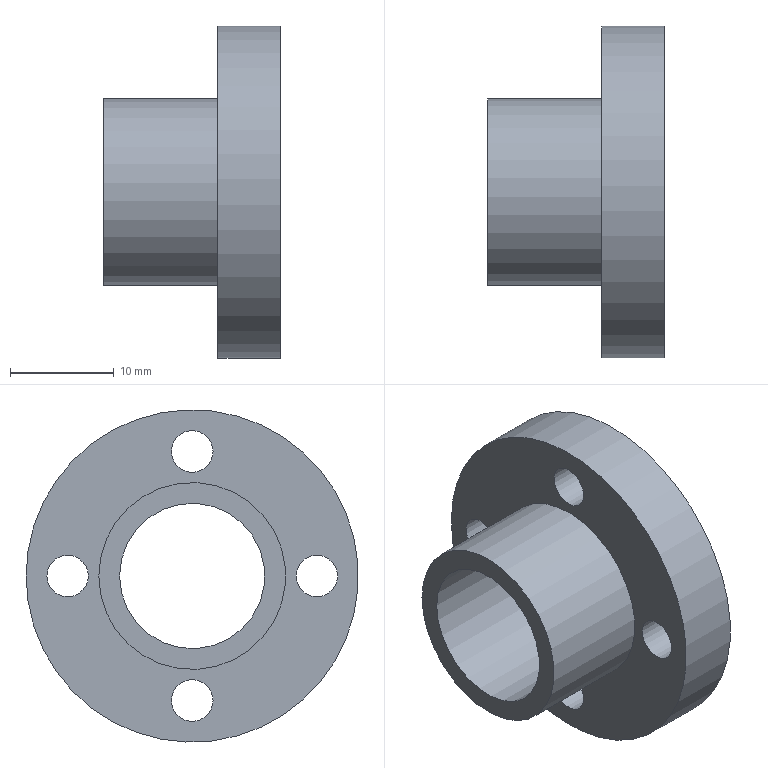Part | STEP file | 1-56.13 | 1 solid | 10 faces | box 17 x 32 x 32 mm | volume 4706 mm3 | cylinder 7 | plane 3 | commonest cylinder face diameters 4 x4 14 x1 18 x1 32 x1
STEP:
#1=CARTESIAN_POINT('',(0.,0.,0.));
#2=DIRECTION('',(0.,0.,1.));
#3=DIRECTION('',(1.,0.,0.));
#4=AXIS2_PLACEMENT_3D('',#1,#2,#3);
#5=CARTESIAN_POINT('',(-11.,9.,0.));
#6=VERTEX_POINT('',#5);
#7=CARTESIAN_POINT('',(-11.,0.,0.));
#8=DIRECTION('',(1.,0.,0.));
#9=DIRECTION('',(0.,1.,0.));
#10=AXIS2_PLACEMENT_3D('',#7,#8,#9);
#11=CIRCLE('',#10,9.);
#12=CARTESIAN_POINT('',(-11.,-2.412,0.));
#13=DIRECTION('',(1.,0.,0.));
#14=DIRECTION('',(0.,0.,-1.));
#15=AXIS2_PLACEMENT_3D('',#12,#13,#14);
#16=PLANE('',#15);
#17=CARTESIAN_POINT('',(0.,2.412));
#18=DIRECTION('',(0.,1.));
#19=AXIS2_PLACEMENT_2D('',#17,#18);
#20=CIRCLE('',#19,9.);
#21=(GEOMETRIC_REPRESENTATION_CONTEXT(2)PARAMETRIC_REPRESENTATION_CONTEXT()REPRESENTATION_CONTEXT('',''));
#22=DEFINITIONAL_REPRESENTATION('',(#20),#21);
#23=PCURVE('',#16,#22);
#24=CARTESIAN_POINT('',(0.,0.,0.));
#25=DIRECTION('',(-1.,0.,0.));
#26=DIRECTION('',(0.,1.,0.));
#27=AXIS2_PLACEMENT_3D('',#24,#25,#26);
#28=CYLINDRICAL_SURFACE('',#27,9.);
#29=CARTESIAN_POINT('',(6.283,11.));
#30=DIRECTION('',(-1.,0.));
#31=VECTOR('',#30,1.);
#32=LINE('',#29,#31);
#33=(GEOMETRIC_REPRESENTATION_CONTEXT(2)PARAMETRIC_REPRESENTATION_CONTEXT()REPRESENTATION_CONTEXT('',''));
#34=DEFINITIONAL_REPRESENTATION('',(#32),#33);
#35=PCURVE('',#28,#34);
#36=SURFACE_CURVE('',#11,(#23,#35),.PCURVE_S1.);
#37=EDGE_CURVE('',#6,#6,#36,.T.);
#38=ORIENTED_EDGE('',*,*,#37,.T.);
#39=EDGE_LOOP('',(#38));
#40=FACE_BOUND('',#39,.F.);
#41=CARTESIAN_POINT('',(-11.,7.,0.));
#42=VERTEX_POINT('',#41);
#43=CARTESIAN_POINT('',(-11.,0.,0.));
#44=DIRECTION('',(-1.,0.,0.));
#45=DIRECTION('',(0.,1.,0.));
#46=AXIS2_PLACEMENT_3D('',#43,#44,#45);
#47=CIRCLE('',#46,7.);
#48=CARTESIAN_POINT('',(0.,9.412));
#49=CARTESIAN_POINT('',(12.124,9.412));
#50=CARTESIAN_POINT('',(6.062,-1.088));
#51=CARTESIAN_POINT('',(0.,-11.588));
#52=CARTESIAN_POINT('',(-6.062,-1.088));
#53=CARTESIAN_POINT('',(-12.124,9.412));
#54=CARTESIAN_POINT('',(0.,9.412));
#55=(BOUNDED_CURVE()B_SPLINE_CURVE(2,(#48,#49,#50,#51,#52,#53,#54),.UNSPECIFIED.,.T.,.F.)B_SPLINE_CURVE_WITH_KNOTS((1,2,2,2,2,1),(-2.094,0.,2.094,4.189,6.283,8.378),.UNSPECIFIED.)CURVE()GEOMETRIC_REPRESENTATION_ITEM()RATIONAL_B_SPLINE_CURVE((1.,0.5,1.,0.5,1.,0.5,1.))REPRESENTATION_ITEM(''));
#56=(GEOMETRIC_REPRESENTATION_CONTEXT(2)PARAMETRIC_REPRESENTATION_CONTEXT()REPRESENTATION_CONTEXT('',''));
#57=DEFINITIONAL_REPRESENTATION('',(#55),#56);
#58=PCURVE('',#16,#57);
#59=CARTESIAN_POINT('',(6.,0.,0.));
#60=DIRECTION('',(-1.,0.,0.));
#61=DIRECTION('',(0.,1.,0.));
#62=AXIS2_PLACEMENT_3D('',#59,#60,#61);
#63=CYLINDRICAL_SURFACE('',#62,7.);
#64=CARTESIAN_POINT('',(0.,17.));
#65=DIRECTION('',(1.,0.));
#66=VECTOR('',#65,1.);
#67=LINE('',#64,#66);
#68=(GEOMETRIC_REPRESENTATION_CONTEXT(2)PARAMETRIC_REPRESENTATION_CONTEXT()REPRESENTATION_CONTEXT('',''));
#69=DEFINITIONAL_REPRESENTATION('',(#67),#68);
#70=PCURVE('',#63,#69);
#71=SURFACE_CURVE('',#47,(#58,#70),.PCURVE_S1.);
#72=EDGE_CURVE('',#42,#42,#71,.T.);
#73=ORIENTED_EDGE('',*,*,#72,.T.);
#74=EDGE_LOOP('',(#73));
#75=FACE_BOUND('',#74,.F.);
#76=ADVANCED_FACE('',(#40,#75),#16,.F.);
#77=CARTESIAN_POINT('',(0.,9.,0.));
#78=VERTEX_POINT('',#77);
#79=CARTESIAN_POINT('',(0.,9.,0.));
#80=DIRECTION('',(-1.,0.,0.));
#81=VECTOR('',#80,1.);
#82=LINE('',#79,#81);
#83=CARTESIAN_POINT('',(6.283,0.));
#84=DIRECTION('',(0.,1.));
#85=VECTOR('',#84,1.);
#86=LINE('',#83,#85);
#87=(GEOMETRIC_REPRESENTATION_CONTEXT(2)PARAMETRIC_REPRESENTATION_CONTEXT()REPRESENTATION_CONTEXT('',''));
#88=DEFINITIONAL_REPRESENTATION('',(#86),#87);
#89=PCURVE('',#28,#88);
#90=CARTESIAN_POINT('',(0.,0.));
#91=DIRECTION('',(0.,1.));
#92=VECTOR('',#91,1.);
#93=LINE('',#90,#92);
#94=(GEOMETRIC_REPRESENTATION_CONTEXT(2)PARAMETRIC_REPRESENTATION_CONTEXT()REPRESENTATION_CONTEXT('',''));
#95=DEFINITIONAL_REPRESENTATION('',(#93),#94);
#96=PCURVE('',#28,#95);
#97=SEAM_CURVE('',#82,(#89,#96),.PCURVE_S1.);
#98=EDGE_CURVE('',#78,#6,#97,.T.);
#99=ORIENTED_EDGE('',*,*,#98,.T.);
#100=ORIENTED_EDGE('',*,*,#37,.T.);
#101=ORIENTED_EDGE('',*,*,#98,.F.);
#102=CARTESIAN_POINT('',(0.,0.,0.));
#103=DIRECTION('',(1.,0.,0.));
#104=DIRECTION('',(0.,1.,0.));
#105=AXIS2_PLACEMENT_3D('',#102,#103,#104);
#106=CIRCLE('',#105,9.);
#107=CARTESIAN_POINT('',(6.283,0.));
#108=DIRECTION('',(-1.,0.));
#109=VECTOR('',#108,1.);
#110=LINE('',#107,#109);
#111=(GEOMETRIC_REPRESENTATION_CONTEXT(2)PARAMETRIC_REPRESENTATION_CONTEXT()REPRESENTATION_CONTEXT('',''));
#112=DEFINITIONAL_REPRESENTATION('',(#110),#111);
#113=PCURVE('',#28,#112);
#114=CARTESIAN_POINT('',(0.,-4.287,0.));
#115=DIRECTION('',(1.,0.,0.));
#116=DIRECTION('',(0.,0.,-1.));
#117=AXIS2_PLACEMENT_3D('',#114,#115,#116);
#118=PLANE('',#117);
#119=CARTESIAN_POINT('',(0.,4.287));
#120=DIRECTION('',(0.,1.));
#121=AXIS2_PLACEMENT_2D('',#119,#120);
#122=CIRCLE('',#121,9.);
#123=(GEOMETRIC_REPRESENTATION_CONTEXT(2)PARAMETRIC_REPRESENTATION_CONTEXT()REPRESENTATION_CONTEXT('',''));
#124=DEFINITIONAL_REPRESENTATION('',(#122),#123);
#125=PCURVE('',#118,#124);
#126=SURFACE_CURVE('',#106,(#113,#125),.PCURVE_S1.);
#127=EDGE_CURVE('',#78,#78,#126,.T.);
#128=ORIENTED_EDGE('',*,*,#127,.F.);
#129=EDGE_LOOP('',(#99,#100,#101,#128));
#130=FACE_BOUND('',#129,.T.);
#131=ADVANCED_FACE('',(#130),#28,.T.);
#132=ORIENTED_EDGE('',*,*,#72,.F.);
#133=CARTESIAN_POINT('',(6.,7.,0.));
#134=VERTEX_POINT('',#133);
#135=CARTESIAN_POINT('',(-11.,7.,0.));
#136=DIRECTION('',(1.,0.,0.));
#137=VECTOR('',#136,1.);
#138=LINE('',#135,#137);
#139=CARTESIAN_POINT('',(0.,17.));
#140=DIRECTION('',(0.,-1.));
#141=VECTOR('',#140,1.);
#142=LINE('',#139,#141);
#143=(GEOMETRIC_REPRESENTATION_CONTEXT(2)PARAMETRIC_REPRESENTATION_CONTEXT()REPRESENTATION_CONTEXT('',''));
#144=DEFINITIONAL_REPRESENTATION('',(#142),#143);
#145=PCURVE('',#63,#144);
#146=CARTESIAN_POINT('',(6.283,17.));
#147=DIRECTION('',(0.,-1.));
#148=VECTOR('',#147,1.);
#149=LINE('',#146,#148);
#150=(GEOMETRIC_REPRESENTATION_CONTEXT(2)PARAMETRIC_REPRESENTATION_CONTEXT()REPRESENTATION_CONTEXT('',''));
#151=DEFINITIONAL_REPRESENTATION('',(#149),#150);
#152=PCURVE('',#63,#151);
#153=SEAM_CURVE('',#138,(#145,#152),.PCURVE_S1.);
#154=EDGE_CURVE('',#42,#134,#153,.T.);
#155=ORIENTED_EDGE('',*,*,#154,.T.);
#156=CARTESIAN_POINT('',(6.,0.,0.));
#157=DIRECTION('',(-1.,0.,0.));
#158=DIRECTION('',(0.,1.,0.));
#159=AXIS2_PLACEMENT_3D('',#156,#157,#158);
#160=CIRCLE('',#159,7.);
#161=CARTESIAN_POINT('',(0.,0.));
#162=DIRECTION('',(1.,0.));
#163=VECTOR('',#162,1.);
#164=LINE('',#161,#163);
#165=(GEOMETRIC_REPRESENTATION_CONTEXT(2)PARAMETRIC_REPRESENTATION_CONTEXT()REPRESENTATION_CONTEXT('',''));
#166=DEFINITIONAL_REPRESENTATION('',(#164),#165);
#167=PCURVE('',#63,#166);
#168=CARTESIAN_POINT('',(6.,-4.287,0.));
#169=DIRECTION('',(1.,0.,0.));
#170=DIRECTION('',(0.,0.,-1.));
#171=AXIS2_PLACEMENT_3D('',#168,#169,#170);
#172=PLANE('',#171);
#173=CARTESIAN_POINT('',(0.,11.287));
#174=CARTESIAN_POINT('',(12.124,11.287));
#175=CARTESIAN_POINT('',(6.062,0.7872));
#176=CARTESIAN_POINT('',(0.,-9.713));
#177=CARTESIAN_POINT('',(-6.062,0.7872));
#178=CARTESIAN_POINT('',(-12.124,11.287));
#179=CARTESIAN_POINT('',(0.,11.287));
#180=(BOUNDED_CURVE()B_SPLINE_CURVE(2,(#173,#174,#175,#176,#177,#178,#179),.UNSPECIFIED.,.T.,.F.)B_SPLINE_CURVE_WITH_KNOTS((1,2,2,2,2,1),(-2.094,0.,2.094,4.189,6.283,8.378),.UNSPECIFIED.)CURVE()GEOMETRIC_REPRESENTATION_ITEM()RATIONAL_B_SPLINE_CURVE((1.,0.5,1.,0.5,1.,0.5,1.))REPRESENTATION_ITEM(''));
#181=(GEOMETRIC_REPRESENTATION_CONTEXT(2)PARAMETRIC_REPRESENTATION_CONTEXT()REPRESENTATION_CONTEXT('',''));
#182=DEFINITIONAL_REPRESENTATION('',(#180),#181);
#183=PCURVE('',#172,#182);
#184=SURFACE_CURVE('',#160,(#167,#183),.PCURVE_S1.);
#185=EDGE_CURVE('',#134,#134,#184,.T.);
#186=ORIENTED_EDGE('',*,*,#185,.T.);
#187=ORIENTED_EDGE('',*,*,#154,.F.);
#188=EDGE_LOOP('',(#132,#155,#186,#187));
#189=FACE_BOUND('',#188,.F.);
#190=ADVANCED_FACE('',(#189),#63,.F.);
#191=CARTESIAN_POINT('',(0.,16.,0.));
#192=VERTEX_POINT('',#191);
#193=CARTESIAN_POINT('',(0.,0.,0.));
#194=DIRECTION('',(1.,0.,0.));
#195=DIRECTION('',(0.,1.,0.));
#196=AXIS2_PLACEMENT_3D('',#193,#194,#195);
#197=CIRCLE('',#196,16.);
#198=CARTESIAN_POINT('',(0.,4.287));
#199=DIRECTION('',(0.,1.));
#200=AXIS2_PLACEMENT_2D('',#198,#199);
#201=CIRCLE('',#200,16.);
#202=(GEOMETRIC_REPRESENTATION_CONTEXT(2)PARAMETRIC_REPRESENTATION_CONTEXT()REPRESENTATION_CONTEXT('',''));
#203=DEFINITIONAL_REPRESENTATION('',(#201),#202);
#204=PCURVE('',#118,#203);
#205=CARTESIAN_POINT('',(0.,0.,0.));
#206=DIRECTION('',(1.,0.,0.));
#207=DIRECTION('',(0.,1.,0.));
#208=AXIS2_PLACEMENT_3D('',#205,#206,#207);
#209=CYLINDRICAL_SURFACE('',#208,16.);
#210=CARTESIAN_POINT('',(0.,0.));
#211=DIRECTION('',(1.,0.));
#212=VECTOR('',#211,1.);
#213=LINE('',#210,#212);
#214=(GEOMETRIC_REPRESENTATION_CONTEXT(2)PARAMETRIC_REPRESENTATION_CONTEXT()REPRESENTATION_CONTEXT('',''));
#215=DEFINITIONAL_REPRESENTATION('',(#213),#214);
#216=PCURVE('',#209,#215);
#217=SURFACE_CURVE('',#197,(#204,#216),.PCURVE_S1.);
#218=EDGE_CURVE('',#192,#192,#217,.T.);
#219=ORIENTED_EDGE('',*,*,#218,.T.);
#220=EDGE_LOOP('',(#219));
#221=FACE_BOUND('',#220,.F.);
#222=ORIENTED_EDGE('',*,*,#127,.F.);
#223=EDGE_LOOP('',(#222));
#224=FACE_BOUND('',#223,.F.);
#225=CARTESIAN_POINT('',(0.,2.,-12.));
#226=VERTEX_POINT('',#225);
#227=CARTESIAN_POINT('',(0.,0.,-12.));
#228=DIRECTION('',(-1.,0.,0.));
#229=DIRECTION('',(0.,1.,0.));
#230=AXIS2_PLACEMENT_3D('',#227,#228,#229);
#231=CIRCLE('',#230,2.);
#232=CARTESIAN_POINT('',(12.,6.287));
#233=CARTESIAN_POINT('',(15.464,6.287));
#234=CARTESIAN_POINT('',(13.732,3.287));
#235=CARTESIAN_POINT('',(12.,0.2872));
#236=CARTESIAN_POINT('',(10.268,3.287));
#237=CARTESIAN_POINT('',(8.536,6.287));
#238=CARTESIAN_POINT('',(12.,6.287));
#239=(BOUNDED_CURVE()B_SPLINE_CURVE(2,(#232,#233,#234,#235,#236,#237,#238),.UNSPECIFIED.,.T.,.F.)B_SPLINE_CURVE_WITH_KNOTS((1,2,2,2,2,1),(-2.094,0.,2.094,4.189,6.283,8.378),.UNSPECIFIED.)CURVE()GEOMETRIC_REPRESENTATION_ITEM()RATIONAL_B_SPLINE_CURVE((1.,0.5,1.,0.5,1.,0.5,1.))REPRESENTATION_ITEM(''));
#240=(GEOMETRIC_REPRESENTATION_CONTEXT(2)PARAMETRIC_REPRESENTATION_CONTEXT()REPRESENTATION_CONTEXT('',''));
#241=DEFINITIONAL_REPRESENTATION('',(#239),#240);
#242=PCURVE('',#118,#241);
#243=CARTESIAN_POINT('',(0.,0.,-12.));
#244=DIRECTION('',(1.,0.,0.));
#245=DIRECTION('',(0.,1.,0.));
#246=AXIS2_PLACEMENT_3D('',#243,#244,#245);
#247=CYLINDRICAL_SURFACE('',#246,2.);
#248=CARTESIAN_POINT('',(6.283,0.));
#249=DIRECTION('',(-1.,0.));
#250=VECTOR('',#249,1.);
#251=LINE('',#248,#250);
#252=(GEOMETRIC_REPRESENTATION_CONTEXT(2)PARAMETRIC_REPRESENTATION_CONTEXT()REPRESENTATION_CONTEXT('',''));
#253=DEFINITIONAL_REPRESENTATION('',(#251),#252);
#254=PCURVE('',#247,#253);
#255=SURFACE_CURVE('',#231,(#242,#254),.PCURVE_S1.);
#256=EDGE_CURVE('',#226,#226,#255,.T.);
#257=ORIENTED_EDGE('',*,*,#256,.T.);
#258=EDGE_LOOP('',(#257));
#259=FACE_BOUND('',#258,.F.);
#260=CARTESIAN_POINT('',(0.,2.,12.));
#261=VERTEX_POINT('',#260);
#262=CARTESIAN_POINT('',(0.,0.,12.));
#263=DIRECTION('',(-1.,0.,0.));
#264=DIRECTION('',(0.,1.,0.));
#265=AXIS2_PLACEMENT_3D('',#262,#263,#264);
#266=CIRCLE('',#265,2.);
#267=CARTESIAN_POINT('',(-12.,6.287));
#268=CARTESIAN_POINT('',(-8.536,6.287));
#269=CARTESIAN_POINT('',(-10.268,3.287));
#270=CARTESIAN_POINT('',(-12.,0.2872));
#271=CARTESIAN_POINT('',(-13.732,3.287));
#272=CARTESIAN_POINT('',(-15.464,6.287));
#273=CARTESIAN_POINT('',(-12.,6.287));
#274=(BOUNDED_CURVE()B_SPLINE_CURVE(2,(#267,#268,#269,#270,#271,#272,#273),.UNSPECIFIED.,.T.,.F.)B_SPLINE_CURVE_WITH_KNOTS((1,2,2,2,2,1),(-2.094,0.,2.094,4.189,6.283,8.378),.UNSPECIFIED.)CURVE()GEOMETRIC_REPRESENTATION_ITEM()RATIONAL_B_SPLINE_CURVE((1.,0.5,1.,0.5,1.,0.5,1.))REPRESENTATION_ITEM(''));
#275=(GEOMETRIC_REPRESENTATION_CONTEXT(2)PARAMETRIC_REPRESENTATION_CONTEXT()REPRESENTATION_CONTEXT('',''));
#276=DEFINITIONAL_REPRESENTATION('',(#274),#275);
#277=PCURVE('',#118,#276);
#278=CARTESIAN_POINT('',(0.,0.,12.));
#279=DIRECTION('',(1.,0.,0.));
#280=DIRECTION('',(0.,1.,0.));
#281=AXIS2_PLACEMENT_3D('',#278,#279,#280);
#282=CYLINDRICAL_SURFACE('',#281,2.);
#283=CARTESIAN_POINT('',(6.283,0.));
#284=DIRECTION('',(-1.,0.));
#285=VECTOR('',#284,1.);
#286=LINE('',#283,#285);
#287=(GEOMETRIC_REPRESENTATION_CONTEXT(2)PARAMETRIC_REPRESENTATION_CONTEXT()REPRESENTATION_CONTEXT('',''));
#288=DEFINITIONAL_REPRESENTATION('',(#286),#287);
#289=PCURVE('',#282,#288);
#290=SURFACE_CURVE('',#266,(#277,#289),.PCURVE_S1.);
#291=EDGE_CURVE('',#261,#261,#290,.T.);
#292=ORIENTED_EDGE('',*,*,#291,.T.);
#293=EDGE_LOOP('',(#292));
#294=FACE_BOUND('',#293,.F.);
#295=CARTESIAN_POINT('',(0.,14.,0.));
#296=VERTEX_POINT('',#295);
#297=CARTESIAN_POINT('',(0.,12.,0.));
#298=DIRECTION('',(-1.,0.,0.));
#299=DIRECTION('',(0.,1.,0.));
#300=AXIS2_PLACEMENT_3D('',#297,#298,#299);
#301=CIRCLE('',#300,2.);
#302=CARTESIAN_POINT('',(0.,18.287));
#303=CARTESIAN_POINT('',(3.464,18.287));
#304=CARTESIAN_POINT('',(1.732,15.287));
#305=CARTESIAN_POINT('',(0.,12.287));
#306=CARTESIAN_POINT('',(-1.732,15.287));
#307=CARTESIAN_POINT('',(-3.464,18.287));
#308=CARTESIAN_POINT('',(0.,18.287));
#309=(BOUNDED_CURVE()B_SPLINE_CURVE(2,(#302,#303,#304,#305,#306,#307,#308),.UNSPECIFIED.,.T.,.F.)B_SPLINE_CURVE_WITH_KNOTS((1,2,2,2,2,1),(-2.094,0.,2.094,4.189,6.283,8.378),.UNSPECIFIED.)CURVE()GEOMETRIC_REPRESENTATION_ITEM()RATIONAL_B_SPLINE_CURVE((1.,0.5,1.,0.5,1.,0.5,1.))REPRESENTATION_ITEM(''));
#310=(GEOMETRIC_REPRESENTATION_CONTEXT(2)PARAMETRIC_REPRESENTATION_CONTEXT()REPRESENTATION_CONTEXT('',''));
#311=DEFINITIONAL_REPRESENTATION('',(#309),#310);
#312=PCURVE('',#118,#311);
#313=CARTESIAN_POINT('',(0.,12.,0.));
#314=DIRECTION('',(1.,0.,0.));
#315=DIRECTION('',(0.,1.,0.));
#316=AXIS2_PLACEMENT_3D('',#313,#314,#315);
#317=CYLINDRICAL_SURFACE('',#316,2.);
#318=CARTESIAN_POINT('',(6.283,0.));
#319=DIRECTION('',(-1.,0.));
#320=VECTOR('',#319,1.);
#321=LINE('',#318,#320);
#322=(GEOMETRIC_REPRESENTATION_CONTEXT(2)PARAMETRIC_REPRESENTATION_CONTEXT()REPRESENTATION_CONTEXT('',''));
#323=DEFINITIONAL_REPRESENTATION('',(#321),#322);
#324=PCURVE('',#317,#323);
#325=SURFACE_CURVE('',#301,(#312,#324),.PCURVE_S1.);
#326=EDGE_CURVE('',#296,#296,#325,.T.);
#327=ORIENTED_EDGE('',*,*,#326,.T.);
#328=EDGE_LOOP('',(#327));
#329=FACE_BOUND('',#328,.F.);
#330=CARTESIAN_POINT('',(0.,-10.,0.));
#331=VERTEX_POINT('',#330);
#332=CARTESIAN_POINT('',(0.,-12.,0.));
#333=DIRECTION('',(-1.,0.,0.));
#334=DIRECTION('',(0.,1.,0.));
#335=AXIS2_PLACEMENT_3D('',#332,#333,#334);
#336=CIRCLE('',#335,2.);
#337=CARTESIAN_POINT('',(0.,-5.713));
#338=CARTESIAN_POINT('',(3.464,-5.713));
#339=CARTESIAN_POINT('',(1.732,-8.713));
#340=CARTESIAN_POINT('',(0.,-11.713));
#341=CARTESIAN_POINT('',(-1.732,-8.713));
#342=CARTESIAN_POINT('',(-3.464,-5.713));
#343=CARTESIAN_POINT('',(0.,-5.713));
#344=(BOUNDED_CURVE()B_SPLINE_CURVE(2,(#337,#338,#339,#340,#341,#342,#343),.UNSPECIFIED.,.T.,.F.)B_SPLINE_CURVE_WITH_KNOTS((1,2,2,2,2,1),(-2.094,0.,2.094,4.189,6.283,8.378),.UNSPECIFIED.)CURVE()GEOMETRIC_REPRESENTATION_ITEM()RATIONAL_B_SPLINE_CURVE((1.,0.5,1.,0.5,1.,0.5,1.))REPRESENTATION_ITEM(''));
#345=(GEOMETRIC_REPRESENTATION_CONTEXT(2)PARAMETRIC_REPRESENTATION_CONTEXT()REPRESENTATION_CONTEXT('',''));
#346=DEFINITIONAL_REPRESENTATION('',(#344),#345);
#347=PCURVE('',#118,#346);
#348=CARTESIAN_POINT('',(0.,-12.,0.));
#349=DIRECTION('',(1.,0.,0.));
#350=DIRECTION('',(0.,1.,0.));
#351=AXIS2_PLACEMENT_3D('',#348,#349,#350);
#352=CYLINDRICAL_SURFACE('',#351,2.);
#353=CARTESIAN_POINT('',(6.283,0.));
#354=DIRECTION('',(-1.,0.));
#355=VECTOR('',#354,1.);
#356=LINE('',#353,#355);
#357=(GEOMETRIC_REPRESENTATION_CONTEXT(2)PARAMETRIC_REPRESENTATION_CONTEXT()REPRESENTATION_CONTEXT('',''));
#358=DEFINITIONAL_REPRESENTATION('',(#356),#357);
#359=PCURVE('',#352,#358);
#360=SURFACE_CURVE('',#336,(#347,#359),.PCURVE_S1.);
#361=EDGE_CURVE('',#331,#331,#360,.T.);
#362=ORIENTED_EDGE('',*,*,#361,.T.);
#363=EDGE_LOOP('',(#362));
#364=FACE_BOUND('',#363,.F.);
#365=ADVANCED_FACE('',(#221,#224,#259,#294,#329,#364),#118,.F.);
#366=ORIENTED_EDGE('',*,*,#218,.T.);
#367=CARTESIAN_POINT('',(6.,16.,0.));
#368=VERTEX_POINT('',#367);
#369=CARTESIAN_POINT('',(0.,16.,0.));
#370=DIRECTION('',(1.,0.,0.));
#371=VECTOR('',#370,1.);
#372=LINE('',#369,#371);
#373=CARTESIAN_POINT('',(6.283,0.));
#374=DIRECTION('',(0.,1.));
#375=VECTOR('',#374,1.);
#376=LINE('',#373,#375);
#377=(GEOMETRIC_REPRESENTATION_CONTEXT(2)PARAMETRIC_REPRESENTATION_CONTEXT()REPRESENTATION_CONTEXT('',''));
#378=DEFINITIONAL_REPRESENTATION('',(#376),#377);
#379=PCURVE('',#209,#378);
#380=CARTESIAN_POINT('',(0.,0.));
#381=DIRECTION('',(0.,1.));
#382=VECTOR('',#381,1.);
#383=LINE('',#380,#382);
#384=(GEOMETRIC_REPRESENTATION_CONTEXT(2)PARAMETRIC_REPRESENTATION_CONTEXT()REPRESENTATION_CONTEXT('',''));
#385=DEFINITIONAL_REPRESENTATION('',(#383),#384);
#386=PCURVE('',#209,#385);
#387=SEAM_CURVE('',#372,(#379,#386),.PCURVE_S1.);
#388=EDGE_CURVE('',#192,#368,#387,.T.);
#389=ORIENTED_EDGE('',*,*,#388,.T.);
#390=CARTESIAN_POINT('',(6.,0.,0.));
#391=DIRECTION('',(1.,0.,0.));
#392=DIRECTION('',(0.,1.,0.));
#393=AXIS2_PLACEMENT_3D('',#390,#391,#392);
#394=CIRCLE('',#393,16.);
#395=CARTESIAN_POINT('',(0.,6.));
#396=DIRECTION('',(1.,0.));
#397=VECTOR('',#396,1.);
#398=LINE('',#395,#397);
#399=(GEOMETRIC_REPRESENTATION_CONTEXT(2)PARAMETRIC_REPRESENTATION_CONTEXT()REPRESENTATION_CONTEXT('',''));
#400=DEFINITIONAL_REPRESENTATION('',(#398),#399);
#401=PCURVE('',#209,#400);
#402=CARTESIAN_POINT('',(0.,4.287));
#403=DIRECTION('',(0.,1.));
#404=AXIS2_PLACEMENT_2D('',#402,#403);
#405=CIRCLE('',#404,16.);
#406=(GEOMETRIC_REPRESENTATION_CONTEXT(2)PARAMETRIC_REPRESENTATION_CONTEXT()REPRESENTATION_CONTEXT('',''));
#407=DEFINITIONAL_REPRESENTATION('',(#405),#406);
#408=PCURVE('',#172,#407);
#409=SURFACE_CURVE('',#394,(#401,#408),.PCURVE_S1.);
#410=EDGE_CURVE('',#368,#368,#409,.T.);
#411=ORIENTED_EDGE('',*,*,#410,.F.);
#412=ORIENTED_EDGE('',*,*,#388,.F.);
#413=EDGE_LOOP('',(#366,#389,#411,#412));
#414=FACE_BOUND('',#413,.T.);
#415=ADVANCED_FACE('',(#414),#209,.T.);
#416=CARTESIAN_POINT('',(6.,2.,-12.));
#417=VERTEX_POINT('',#416);
#418=CARTESIAN_POINT('',(0.,2.,-12.));
#419=DIRECTION('',(1.,0.,0.));
#420=VECTOR('',#419,1.);
#421=LINE('',#418,#420);
#422=CARTESIAN_POINT('',(6.283,0.));
#423=DIRECTION('',(0.,1.));
#424=VECTOR('',#423,1.);
#425=LINE('',#422,#424);
#426=(GEOMETRIC_REPRESENTATION_CONTEXT(2)PARAMETRIC_REPRESENTATION_CONTEXT()REPRESENTATION_CONTEXT('',''));
#427=DEFINITIONAL_REPRESENTATION('',(#425),#426);
#428=PCURVE('',#247,#427);
#429=CARTESIAN_POINT('',(0.,0.));
#430=DIRECTION('',(0.,1.));
#431=VECTOR('',#430,1.);
#432=LINE('',#429,#431);
#433=(GEOMETRIC_REPRESENTATION_CONTEXT(2)PARAMETRIC_REPRESENTATION_CONTEXT()REPRESENTATION_CONTEXT('',''));
#434=DEFINITIONAL_REPRESENTATION('',(#432),#433);
#435=PCURVE('',#247,#434);
#436=SEAM_CURVE('',#421,(#428,#435),.PCURVE_S1.);
#437=EDGE_CURVE('',#226,#417,#436,.T.);
#438=ORIENTED_EDGE('',*,*,#437,.T.);
#439=CARTESIAN_POINT('',(6.,0.,-12.));
#440=DIRECTION('',(-1.,0.,0.));
#441=DIRECTION('',(0.,1.,0.));
#442=AXIS2_PLACEMENT_3D('',#439,#440,#441);
#443=CIRCLE('',#442,2.);
#444=CARTESIAN_POINT('',(6.283,6.));
#445=DIRECTION('',(-1.,0.));
#446=VECTOR('',#445,1.);
#447=LINE('',#444,#446);
#448=(GEOMETRIC_REPRESENTATION_CONTEXT(2)PARAMETRIC_REPRESENTATION_CONTEXT()REPRESENTATION_CONTEXT('',''));
#449=DEFINITIONAL_REPRESENTATION('',(#447),#448);
#450=PCURVE('',#247,#449);
#451=CARTESIAN_POINT('',(12.,6.287));
#452=CARTESIAN_POINT('',(15.464,6.287));
#453=CARTESIAN_POINT('',(13.732,3.287));
#454=CARTESIAN_POINT('',(12.,0.2872));
#455=CARTESIAN_POINT('',(10.268,3.287));
#456=CARTESIAN_POINT('',(8.536,6.287));
#457=CARTESIAN_POINT('',(12.,6.287));
#458=(BOUNDED_CURVE()B_SPLINE_CURVE(2,(#451,#452,#453,#454,#455,#456,#457),.UNSPECIFIED.,.T.,.F.)B_SPLINE_CURVE_WITH_KNOTS((1,2,2,2,2,1),(-2.094,0.,2.094,4.189,6.283,8.378),.UNSPECIFIED.)CURVE()GEOMETRIC_REPRESENTATION_ITEM()RATIONAL_B_SPLINE_CURVE((1.,0.5,1.,0.5,1.,0.5,1.))REPRESENTATION_ITEM(''));
#459=(GEOMETRIC_REPRESENTATION_CONTEXT(2)PARAMETRIC_REPRESENTATION_CONTEXT()REPRESENTATION_CONTEXT('',''));
#460=DEFINITIONAL_REPRESENTATION('',(#458),#459);
#461=PCURVE('',#172,#460);
#462=SURFACE_CURVE('',#443,(#450,#461),.PCURVE_S1.);
#463=EDGE_CURVE('',#417,#417,#462,.T.);
#464=ORIENTED_EDGE('',*,*,#463,.T.);
#465=ORIENTED_EDGE('',*,*,#437,.F.);
#466=ORIENTED_EDGE('',*,*,#256,.F.);
#467=EDGE_LOOP('',(#438,#464,#465,#466));
#468=FACE_BOUND('',#467,.F.);
#469=ADVANCED_FACE('',(#468),#247,.F.);
#470=CARTESIAN_POINT('',(6.,2.,12.));
#471=VERTEX_POINT('',#470);
#472=CARTESIAN_POINT('',(0.,2.,12.));
#473=DIRECTION('',(1.,0.,0.));
#474=VECTOR('',#473,1.);
#475=LINE('',#472,#474);
#476=CARTESIAN_POINT('',(6.283,0.));
#477=DIRECTION('',(0.,1.));
#478=VECTOR('',#477,1.);
#479=LINE('',#476,#478);
#480=(GEOMETRIC_REPRESENTATION_CONTEXT(2)PARAMETRIC_REPRESENTATION_CONTEXT()REPRESENTATION_CONTEXT('',''));
#481=DEFINITIONAL_REPRESENTATION('',(#479),#480);
#482=PCURVE('',#282,#481);
#483=CARTESIAN_POINT('',(0.,0.));
#484=DIRECTION('',(0.,1.));
#485=VECTOR('',#484,1.);
#486=LINE('',#483,#485);
#487=(GEOMETRIC_REPRESENTATION_CONTEXT(2)PARAMETRIC_REPRESENTATION_CONTEXT()REPRESENTATION_CONTEXT('',''));
#488=DEFINITIONAL_REPRESENTATION('',(#486),#487);
#489=PCURVE('',#282,#488);
#490=SEAM_CURVE('',#475,(#482,#489),.PCURVE_S1.);
#491=EDGE_CURVE('',#261,#471,#490,.T.);
#492=ORIENTED_EDGE('',*,*,#491,.T.);
#493=CARTESIAN_POINT('',(6.,0.,12.));
#494=DIRECTION('',(-1.,0.,0.));
#495=DIRECTION('',(0.,1.,0.));
#496=AXIS2_PLACEMENT_3D('',#493,#494,#495);
#497=CIRCLE('',#496,2.);
#498=CARTESIAN_POINT('',(6.283,6.));
#499=DIRECTION('',(-1.,0.));
#500=VECTOR('',#499,1.);
#501=LINE('',#498,#500);
#502=(GEOMETRIC_REPRESENTATION_CONTEXT(2)PARAMETRIC_REPRESENTATION_CONTEXT()REPRESENTATION_CONTEXT('',''));
#503=DEFINITIONAL_REPRESENTATION('',(#501),#502);
#504=PCURVE('',#282,#503);
#505=CARTESIAN_POINT('',(-12.,6.287));
#506=CARTESIAN_POINT('',(-8.536,6.287));
#507=CARTESIAN_POINT('',(-10.268,3.287));
#508=CARTESIAN_POINT('',(-12.,0.2872));
#509=CARTESIAN_POINT('',(-13.732,3.287));
#510=CARTESIAN_POINT('',(-15.464,6.287));
#511=CARTESIAN_POINT('',(-12.,6.287));
#512=(BOUNDED_CURVE()B_SPLINE_CURVE(2,(#505,#506,#507,#508,#509,#510,#511),.UNSPECIFIED.,.T.,.F.)B_SPLINE_CURVE_WITH_KNOTS((1,2,2,2,2,1),(-2.094,0.,2.094,4.189,6.283,8.378),.UNSPECIFIED.)CURVE()GEOMETRIC_REPRESENTATION_ITEM()RATIONAL_B_SPLINE_CURVE((1.,0.5,1.,0.5,1.,0.5,1.))REPRESENTATION_ITEM(''));
#513=(GEOMETRIC_REPRESENTATION_CONTEXT(2)PARAMETRIC_REPRESENTATION_CONTEXT()REPRESENTATION_CONTEXT('',''));
#514=DEFINITIONAL_REPRESENTATION('',(#512),#513);
#515=PCURVE('',#172,#514);
#516=SURFACE_CURVE('',#497,(#504,#515),.PCURVE_S1.);
#517=EDGE_CURVE('',#471,#471,#516,.T.);
#518=ORIENTED_EDGE('',*,*,#517,.T.);
#519=ORIENTED_EDGE('',*,*,#491,.F.);
#520=ORIENTED_EDGE('',*,*,#291,.F.);
#521=EDGE_LOOP('',(#492,#518,#519,#520));
#522=FACE_BOUND('',#521,.F.);
#523=ADVANCED_FACE('',(#522),#282,.F.);
#524=CARTESIAN_POINT('',(6.,14.,0.));
#525=VERTEX_POINT('',#524);
#526=CARTESIAN_POINT('',(0.,14.,0.));
#527=DIRECTION('',(1.,0.,0.));
#528=VECTOR('',#527,1.);
#529=LINE('',#526,#528);
#530=CARTESIAN_POINT('',(6.283,0.));
#531=DIRECTION('',(0.,1.));
#532=VECTOR('',#531,1.);
#533=LINE('',#530,#532);
#534=(GEOMETRIC_REPRESENTATION_CONTEXT(2)PARAMETRIC_REPRESENTATION_CONTEXT()REPRESENTATION_CONTEXT('',''));
#535=DEFINITIONAL_REPRESENTATION('',(#533),#534);
#536=PCURVE('',#317,#535);
#537=CARTESIAN_POINT('',(0.,0.));
#538=DIRECTION('',(0.,1.));
#539=VECTOR('',#538,1.);
#540=LINE('',#537,#539);
#541=(GEOMETRIC_REPRESENTATION_CONTEXT(2)PARAMETRIC_REPRESENTATION_CONTEXT()REPRESENTATION_CONTEXT('',''));
#542=DEFINITIONAL_REPRESENTATION('',(#540),#541);
#543=PCURVE('',#317,#542);
#544=SEAM_CURVE('',#529,(#536,#543),.PCURVE_S1.);
#545=EDGE_CURVE('',#296,#525,#544,.T.);
#546=ORIENTED_EDGE('',*,*,#545,.T.);
#547=CARTESIAN_POINT('',(6.,12.,0.));
#548=DIRECTION('',(-1.,0.,0.));
#549=DIRECTION('',(0.,1.,0.));
#550=AXIS2_PLACEMENT_3D('',#547,#548,#549);
#551=CIRCLE('',#550,2.);
#552=CARTESIAN_POINT('',(6.283,6.));
#553=DIRECTION('',(-1.,0.));
#554=VECTOR('',#553,1.);
#555=LINE('',#552,#554);
#556=(GEOMETRIC_REPRESENTATION_CONTEXT(2)PARAMETRIC_REPRESENTATION_CONTEXT()REPRESENTATION_CONTEXT('',''));
#557=DEFINITIONAL_REPRESENTATION('',(#555),#556);
#558=PCURVE('',#317,#557);
#559=CARTESIAN_POINT('',(0.,18.287));
#560=CARTESIAN_POINT('',(3.464,18.287));
#561=CARTESIAN_POINT('',(1.732,15.287));
#562=CARTESIAN_POINT('',(0.,12.287));
#563=CARTESIAN_POINT('',(-1.732,15.287));
#564=CARTESIAN_POINT('',(-3.464,18.287));
#565=CARTESIAN_POINT('',(0.,18.287));
#566=(BOUNDED_CURVE()B_SPLINE_CURVE(2,(#559,#560,#561,#562,#563,#564,#565),.UNSPECIFIED.,.T.,.F.)B_SPLINE_CURVE_WITH_KNOTS((1,2,2,2,2,1),(-2.094,0.,2.094,4.189,6.283,8.378),.UNSPECIFIED.)CURVE()GEOMETRIC_REPRESENTATION_ITEM()RATIONAL_B_SPLINE_CURVE((1.,0.5,1.,0.5,1.,0.5,1.))REPRESENTATION_ITEM(''));
#567=(GEOMETRIC_REPRESENTATION_CONTEXT(2)PARAMETRIC_REPRESENTATION_CONTEXT()REPRESENTATION_CONTEXT('',''));
#568=DEFINITIONAL_REPRESENTATION('',(#566),#567);
#569=PCURVE('',#172,#568);
#570=SURFACE_CURVE('',#551,(#558,#569),.PCURVE_S1.);
#571=EDGE_CURVE('',#525,#525,#570,.T.);
#572=ORIENTED_EDGE('',*,*,#571,.T.);
#573=ORIENTED_EDGE('',*,*,#545,.F.);
#574=ORIENTED_EDGE('',*,*,#326,.F.);
#575=EDGE_LOOP('',(#546,#572,#573,#574));
#576=FACE_BOUND('',#575,.F.);
#577=ADVANCED_FACE('',(#576),#317,.F.);
#578=CARTESIAN_POINT('',(6.,-10.,0.));
#579=VERTEX_POINT('',#578);
#580=CARTESIAN_POINT('',(0.,-10.,0.));
#581=DIRECTION('',(1.,0.,0.));
#582=VECTOR('',#581,1.);
#583=LINE('',#580,#582);
#584=CARTESIAN_POINT('',(6.283,0.));
#585=DIRECTION('',(0.,1.));
#586=VECTOR('',#585,1.);
#587=LINE('',#584,#586);
#588=(GEOMETRIC_REPRESENTATION_CONTEXT(2)PARAMETRIC_REPRESENTATION_CONTEXT()REPRESENTATION_CONTEXT('',''));
#589=DEFINITIONAL_REPRESENTATION('',(#587),#588);
#590=PCURVE('',#352,#589);
#591=CARTESIAN_POINT('',(0.,0.));
#592=DIRECTION('',(0.,1.));
#593=VECTOR('',#592,1.);
#594=LINE('',#591,#593);
#595=(GEOMETRIC_REPRESENTATION_CONTEXT(2)PARAMETRIC_REPRESENTATION_CONTEXT()REPRESENTATION_CONTEXT('',''));
#596=DEFINITIONAL_REPRESENTATION('',(#594),#595);
#597=PCURVE('',#352,#596);
#598=SEAM_CURVE('',#583,(#590,#597),.PCURVE_S1.);
#599=EDGE_CURVE('',#331,#579,#598,.T.);
#600=ORIENTED_EDGE('',*,*,#599,.T.);
#601=CARTESIAN_POINT('',(6.,-12.,0.));
#602=DIRECTION('',(-1.,0.,0.));
#603=DIRECTION('',(0.,1.,0.));
#604=AXIS2_PLACEMENT_3D('',#601,#602,#603);
#605=CIRCLE('',#604,2.);
#606=CARTESIAN_POINT('',(6.283,6.));
#607=DIRECTION('',(-1.,0.));
#608=VECTOR('',#607,1.);
#609=LINE('',#606,#608);
#610=(GEOMETRIC_REPRESENTATION_CONTEXT(2)PARAMETRIC_REPRESENTATION_CONTEXT()REPRESENTATION_CONTEXT('',''));
#611=DEFINITIONAL_REPRESENTATION('',(#609),#610);
#612=PCURVE('',#352,#611);
#613=CARTESIAN_POINT('',(0.,-5.713));
#614=CARTESIAN_POINT('',(3.464,-5.713));
#615=CARTESIAN_POINT('',(1.732,-8.713));
#616=CARTESIAN_POINT('',(0.,-11.713));
#617=CARTESIAN_POINT('',(-1.732,-8.713));
#618=CARTESIAN_POINT('',(-3.464,-5.713));
#619=CARTESIAN_POINT('',(0.,-5.713));
#620=(BOUNDED_CURVE()B_SPLINE_CURVE(2,(#613,#614,#615,#616,#617,#618,#619),.UNSPECIFIED.,.T.,.F.)B_SPLINE_CURVE_WITH_KNOTS((1,2,2,2,2,1),(-2.094,0.,2.094,4.189,6.283,8.378),.UNSPECIFIED.)CURVE()GEOMETRIC_REPRESENTATION_ITEM()RATIONAL_B_SPLINE_CURVE((1.,0.5,1.,0.5,1.,0.5,1.))REPRESENTATION_ITEM(''));
#621=(GEOMETRIC_REPRESENTATION_CONTEXT(2)PARAMETRIC_REPRESENTATION_CONTEXT()REPRESENTATION_CONTEXT('',''));
#622=DEFINITIONAL_REPRESENTATION('',(#620),#621);
#623=PCURVE('',#172,#622);
#624=SURFACE_CURVE('',#605,(#612,#623),.PCURVE_S1.);
#625=EDGE_CURVE('',#579,#579,#624,.T.);
#626=ORIENTED_EDGE('',*,*,#625,.T.);
#627=ORIENTED_EDGE('',*,*,#599,.F.);
#628=ORIENTED_EDGE('',*,*,#361,.F.);
#629=EDGE_LOOP('',(#600,#626,#627,#628));
#630=FACE_BOUND('',#629,.F.);
#631=ADVANCED_FACE('',(#630),#352,.F.);
#632=ORIENTED_EDGE('',*,*,#410,.T.);
#633=EDGE_LOOP('',(#632));
#634=FACE_BOUND('',#633,.T.);
#635=ORIENTED_EDGE('',*,*,#463,.T.);
#636=EDGE_LOOP('',(#635));
#637=FACE_BOUND('',#636,.T.);
#638=ORIENTED_EDGE('',*,*,#517,.T.);
#639=EDGE_LOOP('',(#638));
#640=FACE_BOUND('',#639,.T.);
#641=ORIENTED_EDGE('',*,*,#185,.T.);
#642=EDGE_LOOP('',(#641));
#643=FACE_BOUND('',#642,.T.);
#644=ORIENTED_EDGE('',*,*,#571,.T.);
#645=EDGE_LOOP('',(#644));
#646=FACE_BOUND('',#645,.T.);
#647=ORIENTED_EDGE('',*,*,#625,.T.);
#648=EDGE_LOOP('',(#647));
#649=FACE_BOUND('',#648,.T.);
#650=ADVANCED_FACE('',(#634,#637,#640,#643,#646,#649),#172,.T.);
#651=CLOSED_SHELL('',(#76,#131,#190,#365,#415,#469,#523,#577,#631,#650));
#652=MANIFOLD_SOLID_BREP('',#651);
#653=(LENGTH_UNIT()NAMED_UNIT(*)SI_UNIT(.MILLI.,.METRE.));
#654=UNCERTAINTY_MEASURE_WITH_UNIT(LENGTH_MEASURE(0.0000001),#653,'','');
#655=(NAMED_UNIT(*)PLANE_ANGLE_UNIT()SI_UNIT($,.RADIAN.));
#656=(NAMED_UNIT(*)SI_UNIT($,.STERADIAN.)SOLID_ANGLE_UNIT());
#657=(GEOMETRIC_REPRESENTATION_CONTEXT(3)GLOBAL_UNCERTAINTY_ASSIGNED_CONTEXT((#654))GLOBAL_UNIT_ASSIGNED_CONTEXT((#653,#655,#656))REPRESENTATION_CONTEXT('',''));
#658=ADVANCED_BREP_SHAPE_REPRESENTATION('',(#4,#652),#657);